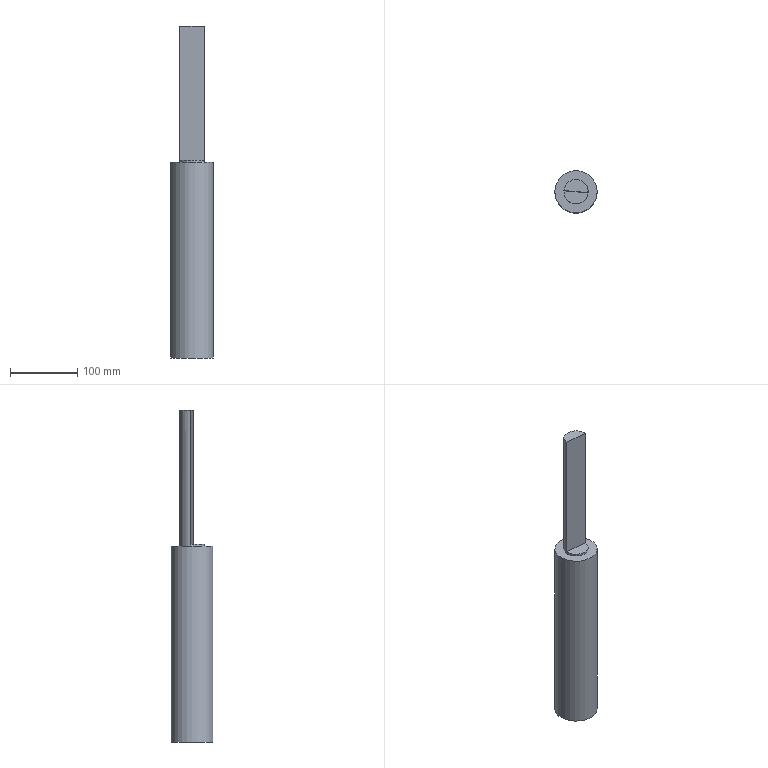Part | NX | features solid 2 | 1 solid | 7 faces | box 63 x 63 x 495 mm | volume 1015077 mm3 | plane 5 | cylinder 2 | commonest cylinder face diameters 36 x1 63 x1
STEP:
#1=CARTESIAN_POINT('',(232.144,308.142,-328.));
#2=VERTEX_POINT('',#1);
#3=CARTESIAN_POINT('',(200.644,308.142,-328.));
#4=DIRECTION('',(0.,0.,1.));
#5=DIRECTION('',(1.,0.,0.));
#6=AXIS2_PLACEMENT_3D('',#3,#4,#5);
#7=CIRCLE('',#6,31.5);
#8=EDGE_CURVE('',#2,#2,#7,.T.);
#9=ORIENTED_EDGE('',*,*,#8,.T.);
#10=EDGE_LOOP('',(#9));
#11=FACE_BOUND('',#10,.T.);
#12=CARTESIAN_POINT('',(218.644,308.142,-328.));
#13=VERTEX_POINT('',#12);
#14=CARTESIAN_POINT('',(200.644,308.142,-328.));
#15=DIRECTION('',(0.,0.,1.));
#16=DIRECTION('',(1.,0.,0.));
#17=AXIS2_PLACEMENT_3D('',#14,#15,#16);
#18=CIRCLE('',#17,18.);
#19=EDGE_CURVE('',#13,#13,#18,.T.);
#20=ORIENTED_EDGE('',*,*,#19,.F.);
#21=EDGE_LOOP('',(#20));
#22=FACE_BOUND('',#21,.T.);
#23=CARTESIAN_POINT('',(200.644,308.142,-328.));
#24=DIRECTION('',(0.,0.,1.));
#25=DIRECTION('',(1.,0.,0.));
#26=AXIS2_PLACEMENT_3D('',#23,#24,#25);
#27=PLANE('',#26);
#28=ADVANCED_FACE('',(#11,#22),#27,.T.);
#29=CARTESIAN_POINT('',(232.144,308.142,-620.));
#30=VERTEX_POINT('',#29);
#31=CARTESIAN_POINT('',(200.644,308.142,-620.));
#32=DIRECTION('',(0.,0.,1.));
#33=DIRECTION('',(1.,0.,0.));
#34=AXIS2_PLACEMENT_3D('',#31,#32,#33);
#35=CIRCLE('',#34,31.5);
#36=EDGE_CURVE('',#30,#30,#35,.T.);
#37=ORIENTED_EDGE('',*,*,#36,.T.);
#38=EDGE_LOOP('',(#37));
#39=FACE_BOUND('',#38,.T.);
#40=ORIENTED_EDGE('',*,*,#8,.F.);
#41=EDGE_LOOP('',(#40));
#42=FACE_BOUND('',#41,.T.);
#43=CARTESIAN_POINT('',(200.644,308.142,-620.));
#44=DIRECTION('',(0.,0.,1.));
#45=DIRECTION('',(1.,0.,0.));
#46=AXIS2_PLACEMENT_3D('',#43,#44,#45);
#47=CYLINDRICAL_SURFACE('',#46,31.5);
#48=ADVANCED_FACE('',(#39,#42),#47,.T.);
#49=ORIENTED_EDGE('',*,*,#36,.F.);
#50=EDGE_LOOP('',(#49));
#51=FACE_BOUND('',#50,.T.);
#52=CARTESIAN_POINT('',(200.644,308.142,-620.));
#53=DIRECTION('',(0.,0.,1.));
#54=DIRECTION('',(1.,0.,0.));
#55=AXIS2_PLACEMENT_3D('',#52,#53,#54);
#56=PLANE('',#55);
#57=ADVANCED_FACE('',(#51),#56,.F.);
#58=CARTESIAN_POINT('',(182.712,309.711,-325.));
#59=VERTEX_POINT('',#58);
#60=CARTESIAN_POINT('',(218.575,306.573,-325.));
#61=VERTEX_POINT('',#60);
#62=CARTESIAN_POINT('',(200.644,308.142,-325.));
#63=DIRECTION('',(0.,0.,1.));
#64=DIRECTION('',(1.,0.,0.));
#65=AXIS2_PLACEMENT_3D('',#62,#63,#64);
#66=CIRCLE('',#65,18.);
#67=EDGE_CURVE('',#59,#61,#66,.T.);
#68=ORIENTED_EDGE('',*,*,#67,.F.);
#69=CARTESIAN_POINT('',(182.712,309.711,-125.));
#70=VERTEX_POINT('',#69);
#71=CARTESIAN_POINT('',(182.712,309.711,-125.));
#72=DIRECTION('',(0.,0.,-1.));
#73=VECTOR('',#72,1000.);
#74=LINE('',#71,#73);
#75=EDGE_CURVE('',#70,#59,#74,.T.);
#76=ORIENTED_EDGE('',*,*,#75,.F.);
#77=CARTESIAN_POINT('',(218.575,306.573,-125.));
#78=VERTEX_POINT('',#77);
#79=CARTESIAN_POINT('',(200.644,308.142,-125.));
#80=DIRECTION('',(0.,0.,1.));
#81=DIRECTION('',(1.,0.,0.));
#82=AXIS2_PLACEMENT_3D('',#79,#80,#81);
#83=CIRCLE('',#82,18.);
#84=EDGE_CURVE('',#78,#70,#83,.T.);
#85=ORIENTED_EDGE('',*,*,#84,.F.);
#86=CARTESIAN_POINT('',(218.575,306.573,-125.));
#87=DIRECTION('',(0.,0.,-1.));
#88=VECTOR('',#87,1000.);
#89=LINE('',#86,#88);
#90=EDGE_CURVE('',#61,#78,#89,.F.);
#91=ORIENTED_EDGE('',*,*,#90,.F.);
#92=EDGE_LOOP('',(#68,#76,#85,#91));
#93=FACE_BOUND('',#92,.T.);
#94=ORIENTED_EDGE('',*,*,#19,.T.);
#95=EDGE_LOOP('',(#94));
#96=FACE_BOUND('',#95,.T.);
#97=CARTESIAN_POINT('',(200.644,308.142,-325.));
#98=DIRECTION('',(0.,0.,-1.));
#99=DIRECTION('',(-1.,0.,0.));
#100=AXIS2_PLACEMENT_3D('',#97,#98,#99);
#101=CYLINDRICAL_SURFACE('',#100,18.);
#102=ADVANCED_FACE('',(#93,#96),#101,.T.);
#103=CARTESIAN_POINT('',(200.644,308.142,-325.));
#104=DIRECTION('',(0.9962,-0.08716,0.));
#105=VECTOR('',#104,1000.);
#106=LINE('',#103,#105);
#107=EDGE_CURVE('',#59,#61,#106,.T.);
#108=ORIENTED_EDGE('',*,*,#107,.F.);
#109=ORIENTED_EDGE('',*,*,#67,.T.);
#110=EDGE_LOOP('',(#108,#109));
#111=FACE_BOUND('',#110,.T.);
#112=CARTESIAN_POINT('',(200.644,308.142,-325.));
#113=DIRECTION('',(0.,0.,1.));
#114=DIRECTION('',(1.,0.,0.));
#115=AXIS2_PLACEMENT_3D('',#112,#113,#114);
#116=PLANE('',#115);
#117=ADVANCED_FACE('',(#111),#116,.T.);
#118=ORIENTED_EDGE('',*,*,#84,.T.);
#119=CARTESIAN_POINT('',(200.644,308.142,-125.));
#120=DIRECTION('',(0.9962,-0.08716,0.));
#121=VECTOR('',#120,1000.);
#122=LINE('',#119,#121);
#123=EDGE_CURVE('',#70,#78,#122,.T.);
#124=ORIENTED_EDGE('',*,*,#123,.T.);
#125=EDGE_LOOP('',(#118,#124));
#126=FACE_BOUND('',#125,.T.);
#127=CARTESIAN_POINT('',(200.644,308.142,-125.));
#128=DIRECTION('',(0.,0.,1.));
#129=DIRECTION('',(1.,0.,0.));
#130=AXIS2_PLACEMENT_3D('',#127,#128,#129);
#131=PLANE('',#130);
#132=ADVANCED_FACE('',(#126),#131,.T.);
#133=ORIENTED_EDGE('',*,*,#123,.F.);
#134=ORIENTED_EDGE('',*,*,#75,.T.);
#135=ORIENTED_EDGE('',*,*,#107,.T.);
#136=ORIENTED_EDGE('',*,*,#90,.T.);
#137=EDGE_LOOP('',(#133,#134,#135,#136));
#138=FACE_BOUND('',#137,.T.);
#139=CARTESIAN_POINT('',(188.202,309.231,-125.));
#140=DIRECTION('',(-0.08716,-0.9962,0.));
#141=DIRECTION('',(0.9962,-0.08716,0.));
#142=AXIS2_PLACEMENT_3D('',#139,#140,#141);
#143=PLANE('',#142);
#144=ADVANCED_FACE('',(#138),#143,.T.);
#145=CLOSED_SHELL('',(#28,#48,#57,#102,#117,#132,#144));
#146=MANIFOLD_SOLID_BREP('',#145);
#147=(LENGTH_UNIT()NAMED_UNIT(*)SI_UNIT(.MILLI.,.METRE.));
#148=UNCERTAINTY_MEASURE_WITH_UNIT(LENGTH_MEASURE(0.00001),#147,'','');
#149=(NAMED_UNIT(*)PLANE_ANGLE_UNIT()SI_UNIT($,.RADIAN.));
#150=(NAMED_UNIT(*)SI_UNIT($,.STERADIAN.)SOLID_ANGLE_UNIT());
#151=(GEOMETRIC_REPRESENTATION_CONTEXT(3)GLOBAL_UNCERTAINTY_ASSIGNED_CONTEXT((#148))GLOBAL_UNIT_ASSIGNED_CONTEXT((#147,#149,#150))REPRESENTATION_CONTEXT('',''));
#152=ADVANCED_BREP_SHAPE_REPRESENTATION('',(#146),#151);